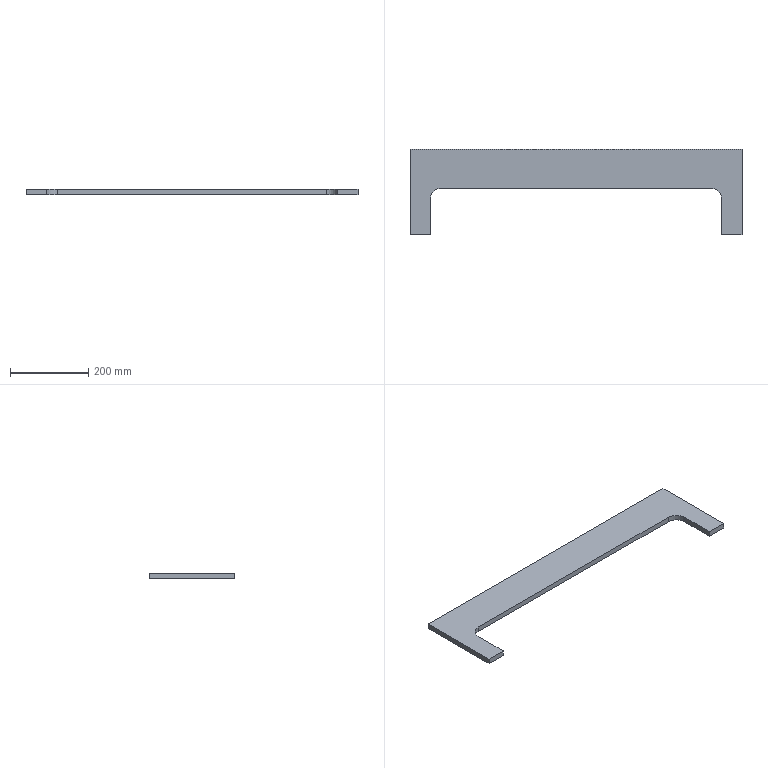Part | STEP file | 2012-06-08-04 | 1 solid | 12 faces | box 850 x 220 x 14 mm | volume 1368448 mm3 | plane 10 | cylinder 2 | commonest cylinder face diameters 60 x2
STEP:
#1=CARTESIAN_POINT('',(0.,0.,0.));
#2=DIRECTION('',(0.,0.,1.));
#3=DIRECTION('',(1.,0.,0.));
#4=AXIS2_PLACEMENT_3D('',#1,#2,#3);
#5=CARTESIAN_POINT('',(-425.,-110.,0.));
#6=VERTEX_POINT('',#5);
#7=CARTESIAN_POINT('',(-373.5,-110.,0.));
#8=VERTEX_POINT('',#7);
#9=CARTESIAN_POINT('',(-425.,-110.,0.));
#10=DIRECTION('',(1.,0.,0.));
#11=VECTOR('',#10,1.);
#12=LINE('',#9,#11);
#13=CARTESIAN_POINT('',(-425.,-110.,14.));
#14=DIRECTION('',(0.,1.,0.));
#15=DIRECTION('',(0.,0.,1.));
#16=AXIS2_PLACEMENT_3D('',#13,#14,#15);
#17=PLANE('',#16);
#18=CARTESIAN_POINT('',(-14.,0.));
#19=DIRECTION('',(0.,1.));
#20=VECTOR('',#19,1.);
#21=LINE('',#18,#20);
#22=(GEOMETRIC_REPRESENTATION_CONTEXT(2)PARAMETRIC_REPRESENTATION_CONTEXT()REPRESENTATION_CONTEXT('',''));
#23=DEFINITIONAL_REPRESENTATION('',(#21),#22);
#24=PCURVE('',#17,#23);
#25=CARTESIAN_POINT('',(425.,-110.,0.));
#26=DIRECTION('',(0.,0.,1.));
#27=DIRECTION('',(1.,0.,0.));
#28=AXIS2_PLACEMENT_3D('',#25,#26,#27);
#29=PLANE('',#28);
#30=CARTESIAN_POINT('',(-850.,0.));
#31=DIRECTION('',(1.,0.));
#32=VECTOR('',#31,1.);
#33=LINE('',#30,#32);
#34=(GEOMETRIC_REPRESENTATION_CONTEXT(2)PARAMETRIC_REPRESENTATION_CONTEXT()REPRESENTATION_CONTEXT('',''));
#35=DEFINITIONAL_REPRESENTATION('',(#33),#34);
#36=PCURVE('',#29,#35);
#37=SURFACE_CURVE('',#12,(#24,#36),.PCURVE_S1.);
#38=EDGE_CURVE('',#6,#8,#37,.T.);
#39=ORIENTED_EDGE('',*,*,#38,.T.);
#40=CARTESIAN_POINT('',(-373.5,-110.,14.));
#41=VERTEX_POINT('',#40);
#42=CARTESIAN_POINT('',(-373.5,-110.,0.));
#43=DIRECTION('',(0.,0.,1.));
#44=VECTOR('',#43,1.);
#45=LINE('',#42,#44);
#46=CARTESIAN_POINT('',(-14.,51.5));
#47=DIRECTION('',(1.,0.));
#48=VECTOR('',#47,1.);
#49=LINE('',#46,#48);
#50=(GEOMETRIC_REPRESENTATION_CONTEXT(2)PARAMETRIC_REPRESENTATION_CONTEXT()REPRESENTATION_CONTEXT('',''));
#51=DEFINITIONAL_REPRESENTATION('',(#49),#50);
#52=PCURVE('',#17,#51);
#53=CARTESIAN_POINT('',(-373.5,-110.,0.));
#54=DIRECTION('',(-1.,0.,0.));
#55=DIRECTION('',(0.,0.,1.));
#56=AXIS2_PLACEMENT_3D('',#53,#54,#55);
#57=PLANE('',#56);
#58=CARTESIAN_POINT('',(0.,0.));
#59=DIRECTION('',(1.,0.));
#60=VECTOR('',#59,1.);
#61=LINE('',#58,#60);
#62=(GEOMETRIC_REPRESENTATION_CONTEXT(2)PARAMETRIC_REPRESENTATION_CONTEXT()REPRESENTATION_CONTEXT('',''));
#63=DEFINITIONAL_REPRESENTATION('',(#61),#62);
#64=PCURVE('',#57,#63);
#65=SURFACE_CURVE('',#45,(#52,#64),.PCURVE_S1.);
#66=EDGE_CURVE('',#8,#41,#65,.T.);
#67=ORIENTED_EDGE('',*,*,#66,.T.);
#68=CARTESIAN_POINT('',(-425.,-110.,14.));
#69=VERTEX_POINT('',#68);
#70=CARTESIAN_POINT('',(-425.,-110.,14.));
#71=DIRECTION('',(1.,0.,0.));
#72=VECTOR('',#71,1.);
#73=LINE('',#70,#72);
#74=CARTESIAN_POINT('',(0.,0.));
#75=DIRECTION('',(0.,1.));
#76=VECTOR('',#75,1.);
#77=LINE('',#74,#76);
#78=(GEOMETRIC_REPRESENTATION_CONTEXT(2)PARAMETRIC_REPRESENTATION_CONTEXT()REPRESENTATION_CONTEXT('',''));
#79=DEFINITIONAL_REPRESENTATION('',(#77),#78);
#80=PCURVE('',#17,#79);
#81=CARTESIAN_POINT('',(425.,-110.,14.));
#82=DIRECTION('',(0.,0.,1.));
#83=DIRECTION('',(1.,0.,0.));
#84=AXIS2_PLACEMENT_3D('',#81,#82,#83);
#85=PLANE('',#84);
#86=CARTESIAN_POINT('',(-850.,0.));
#87=DIRECTION('',(1.,0.));
#88=VECTOR('',#87,1.);
#89=LINE('',#86,#88);
#90=(GEOMETRIC_REPRESENTATION_CONTEXT(2)PARAMETRIC_REPRESENTATION_CONTEXT()REPRESENTATION_CONTEXT('',''));
#91=DEFINITIONAL_REPRESENTATION('',(#89),#90);
#92=PCURVE('',#85,#91);
#93=SURFACE_CURVE('',#73,(#80,#92),.PCURVE_S1.);
#94=EDGE_CURVE('',#69,#41,#93,.T.);
#95=ORIENTED_EDGE('',*,*,#94,.F.);
#96=CARTESIAN_POINT('',(-425.,-110.,14.));
#97=DIRECTION('',(0.,0.,-1.));
#98=VECTOR('',#97,1.);
#99=LINE('',#96,#98);
#100=CARTESIAN_POINT('',(0.,0.));
#101=DIRECTION('',(-1.,0.));
#102=VECTOR('',#101,1.);
#103=LINE('',#100,#102);
#104=(GEOMETRIC_REPRESENTATION_CONTEXT(2)PARAMETRIC_REPRESENTATION_CONTEXT()REPRESENTATION_CONTEXT('',''));
#105=DEFINITIONAL_REPRESENTATION('',(#103),#104);
#106=PCURVE('',#17,#105);
#107=CARTESIAN_POINT('',(-425.,110.,14.));
#108=DIRECTION('',(1.,0.,0.));
#109=DIRECTION('',(0.,1.,0.));
#110=AXIS2_PLACEMENT_3D('',#107,#108,#109);
#111=PLANE('',#110);
#112=CARTESIAN_POINT('',(-220.,0.));
#113=DIRECTION('',(0.,-1.));
#114=VECTOR('',#113,1.);
#115=LINE('',#112,#114);
#116=(GEOMETRIC_REPRESENTATION_CONTEXT(2)PARAMETRIC_REPRESENTATION_CONTEXT()REPRESENTATION_CONTEXT('',''));
#117=DEFINITIONAL_REPRESENTATION('',(#115),#116);
#118=PCURVE('',#111,#117);
#119=SURFACE_CURVE('',#99,(#106,#118),.PCURVE_S1.);
#120=EDGE_CURVE('',#69,#6,#119,.T.);
#121=ORIENTED_EDGE('',*,*,#120,.T.);
#122=EDGE_LOOP('',(#39,#67,#95,#121));
#123=FACE_BOUND('',#122,.T.);
#124=ADVANCED_FACE('',(#123),#17,.F.);
#125=CARTESIAN_POINT('',(425.,-110.,0.));
#126=VERTEX_POINT('',#125);
#127=CARTESIAN_POINT('',(425.,110.,0.));
#128=VERTEX_POINT('',#127);
#129=CARTESIAN_POINT('',(425.,110.,0.));
#130=DIRECTION('',(0.,1.,0.));
#131=VECTOR('',#130,1.);
#132=LINE('',#129,#131);
#133=CARTESIAN_POINT('',(425.,110.,14.));
#134=DIRECTION('',(-1.,0.,0.));
#135=DIRECTION('',(0.,0.,1.));
#136=AXIS2_PLACEMENT_3D('',#133,#134,#135);
#137=PLANE('',#136);
#138=CARTESIAN_POINT('',(-14.,0.));
#139=DIRECTION('',(0.,1.));
#140=VECTOR('',#139,1.);
#141=LINE('',#138,#140);
#142=(GEOMETRIC_REPRESENTATION_CONTEXT(2)PARAMETRIC_REPRESENTATION_CONTEXT()REPRESENTATION_CONTEXT('',''));
#143=DEFINITIONAL_REPRESENTATION('',(#141),#142);
#144=PCURVE('',#137,#143);
#145=CARTESIAN_POINT('',(0.,220.));
#146=DIRECTION('',(0.,1.));
#147=VECTOR('',#146,1.);
#148=LINE('',#145,#147);
#149=(GEOMETRIC_REPRESENTATION_CONTEXT(2)PARAMETRIC_REPRESENTATION_CONTEXT()REPRESENTATION_CONTEXT('',''));
#150=DEFINITIONAL_REPRESENTATION('',(#148),#149);
#151=PCURVE('',#29,#150);
#152=SURFACE_CURVE('',#132,(#144,#151),.PCURVE_S1.);
#153=EDGE_CURVE('',#126,#128,#152,.T.);
#154=ORIENTED_EDGE('',*,*,#153,.T.);
#155=CARTESIAN_POINT('',(425.,110.,14.));
#156=VERTEX_POINT('',#155);
#157=CARTESIAN_POINT('',(425.,110.,14.));
#158=DIRECTION('',(0.,0.,-1.));
#159=VECTOR('',#158,1.);
#160=LINE('',#157,#159);
#161=CARTESIAN_POINT('',(0.,0.));
#162=DIRECTION('',(-1.,0.));
#163=VECTOR('',#162,1.);
#164=LINE('',#161,#163);
#165=(GEOMETRIC_REPRESENTATION_CONTEXT(2)PARAMETRIC_REPRESENTATION_CONTEXT()REPRESENTATION_CONTEXT('',''));
#166=DEFINITIONAL_REPRESENTATION('',(#164),#165);
#167=PCURVE('',#137,#166);
#168=CARTESIAN_POINT('',(-425.,110.,14.));
#169=DIRECTION('',(0.,-1.,0.));
#170=DIRECTION('',(0.,0.,-1.));
#171=AXIS2_PLACEMENT_3D('',#168,#169,#170);
#172=PLANE('',#171);
#173=CARTESIAN_POINT('',(0.,850.));
#174=DIRECTION('',(1.,0.));
#175=VECTOR('',#174,1.);
#176=LINE('',#173,#175);
#177=(GEOMETRIC_REPRESENTATION_CONTEXT(2)PARAMETRIC_REPRESENTATION_CONTEXT()REPRESENTATION_CONTEXT('',''));
#178=DEFINITIONAL_REPRESENTATION('',(#176),#177);
#179=PCURVE('',#172,#178);
#180=SURFACE_CURVE('',#160,(#167,#179),.PCURVE_S1.);
#181=EDGE_CURVE('',#156,#128,#180,.T.);
#182=ORIENTED_EDGE('',*,*,#181,.F.);
#183=CARTESIAN_POINT('',(425.,-110.,14.));
#184=VERTEX_POINT('',#183);
#185=CARTESIAN_POINT('',(425.,110.,14.));
#186=DIRECTION('',(0.,1.,0.));
#187=VECTOR('',#186,1.);
#188=LINE('',#185,#187);
#189=CARTESIAN_POINT('',(0.,0.));
#190=DIRECTION('',(0.,1.));
#191=VECTOR('',#190,1.);
#192=LINE('',#189,#191);
#193=(GEOMETRIC_REPRESENTATION_CONTEXT(2)PARAMETRIC_REPRESENTATION_CONTEXT()REPRESENTATION_CONTEXT('',''));
#194=DEFINITIONAL_REPRESENTATION('',(#192),#193);
#195=PCURVE('',#137,#194);
#196=CARTESIAN_POINT('',(0.,220.));
#197=DIRECTION('',(0.,1.));
#198=VECTOR('',#197,1.);
#199=LINE('',#196,#198);
#200=(GEOMETRIC_REPRESENTATION_CONTEXT(2)PARAMETRIC_REPRESENTATION_CONTEXT()REPRESENTATION_CONTEXT('',''));
#201=DEFINITIONAL_REPRESENTATION('',(#199),#200);
#202=PCURVE('',#85,#201);
#203=SURFACE_CURVE('',#188,(#195,#202),.PCURVE_S1.);
#204=EDGE_CURVE('',#184,#156,#203,.T.);
#205=ORIENTED_EDGE('',*,*,#204,.F.);
#206=CARTESIAN_POINT('',(425.,-110.,14.));
#207=DIRECTION('',(0.,0.,-1.));
#208=VECTOR('',#207,1.);
#209=LINE('',#206,#208);
#210=CARTESIAN_POINT('',(0.,-220.));
#211=DIRECTION('',(-1.,0.));
#212=VECTOR('',#211,1.);
#213=LINE('',#210,#212);
#214=(GEOMETRIC_REPRESENTATION_CONTEXT(2)PARAMETRIC_REPRESENTATION_CONTEXT()REPRESENTATION_CONTEXT('',''));
#215=DEFINITIONAL_REPRESENTATION('',(#213),#214);
#216=PCURVE('',#137,#215);
#217=CARTESIAN_POINT('',(-425.,-110.,14.));
#218=DIRECTION('',(0.,1.,0.));
#219=DIRECTION('',(0.,0.,1.));
#220=AXIS2_PLACEMENT_3D('',#217,#218,#219);
#221=PLANE('',#220);
#222=CARTESIAN_POINT('',(0.,850.));
#223=DIRECTION('',(-1.,0.));
#224=VECTOR('',#223,1.);
#225=LINE('',#222,#224);
#226=(GEOMETRIC_REPRESENTATION_CONTEXT(2)PARAMETRIC_REPRESENTATION_CONTEXT()REPRESENTATION_CONTEXT('',''));
#227=DEFINITIONAL_REPRESENTATION('',(#225),#226);
#228=PCURVE('',#221,#227);
#229=SURFACE_CURVE('',#209,(#216,#228),.PCURVE_S1.);
#230=EDGE_CURVE('',#184,#126,#229,.T.);
#231=ORIENTED_EDGE('',*,*,#230,.T.);
#232=EDGE_LOOP('',(#154,#182,#205,#231));
#233=FACE_BOUND('',#232,.T.);
#234=ADVANCED_FACE('',(#233),#137,.F.);
#235=CARTESIAN_POINT('',(-425.,110.,0.));
#236=VERTEX_POINT('',#235);
#237=CARTESIAN_POINT('',(-425.,110.,0.));
#238=DIRECTION('',(-1.,0.,0.));
#239=VECTOR('',#238,1.);
#240=LINE('',#237,#239);
#241=CARTESIAN_POINT('',(14.,0.));
#242=DIRECTION('',(0.,-1.));
#243=VECTOR('',#242,1.);
#244=LINE('',#241,#243);
#245=(GEOMETRIC_REPRESENTATION_CONTEXT(2)PARAMETRIC_REPRESENTATION_CONTEXT()REPRESENTATION_CONTEXT('',''));
#246=DEFINITIONAL_REPRESENTATION('',(#244),#245);
#247=PCURVE('',#172,#246);
#248=CARTESIAN_POINT('',(-850.,220.));
#249=DIRECTION('',(-1.,0.));
#250=VECTOR('',#249,1.);
#251=LINE('',#248,#250);
#252=(GEOMETRIC_REPRESENTATION_CONTEXT(2)PARAMETRIC_REPRESENTATION_CONTEXT()REPRESENTATION_CONTEXT('',''));
#253=DEFINITIONAL_REPRESENTATION('',(#251),#252);
#254=PCURVE('',#29,#253);
#255=SURFACE_CURVE('',#240,(#247,#254),.PCURVE_S1.);
#256=EDGE_CURVE('',#128,#236,#255,.T.);
#257=ORIENTED_EDGE('',*,*,#256,.T.);
#258=CARTESIAN_POINT('',(-425.,110.,14.));
#259=VERTEX_POINT('',#258);
#260=CARTESIAN_POINT('',(-425.,110.,14.));
#261=DIRECTION('',(0.,0.,-1.));
#262=VECTOR('',#261,1.);
#263=LINE('',#260,#262);
#264=CARTESIAN_POINT('',(0.,0.));
#265=DIRECTION('',(1.,0.));
#266=VECTOR('',#265,1.);
#267=LINE('',#264,#266);
#268=(GEOMETRIC_REPRESENTATION_CONTEXT(2)PARAMETRIC_REPRESENTATION_CONTEXT()REPRESENTATION_CONTEXT('',''));
#269=DEFINITIONAL_REPRESENTATION('',(#267),#268);
#270=PCURVE('',#172,#269);
#271=CARTESIAN_POINT('',(0.,0.));
#272=DIRECTION('',(0.,-1.));
#273=VECTOR('',#272,1.);
#274=LINE('',#271,#273);
#275=(GEOMETRIC_REPRESENTATION_CONTEXT(2)PARAMETRIC_REPRESENTATION_CONTEXT()REPRESENTATION_CONTEXT('',''));
#276=DEFINITIONAL_REPRESENTATION('',(#274),#275);
#277=PCURVE('',#111,#276);
#278=SURFACE_CURVE('',#263,(#270,#277),.PCURVE_S1.);
#279=EDGE_CURVE('',#259,#236,#278,.T.);
#280=ORIENTED_EDGE('',*,*,#279,.F.);
#281=CARTESIAN_POINT('',(-425.,110.,14.));
#282=DIRECTION('',(-1.,0.,0.));
#283=VECTOR('',#282,1.);
#284=LINE('',#281,#283);
#285=CARTESIAN_POINT('',(0.,0.));
#286=DIRECTION('',(0.,-1.));
#287=VECTOR('',#286,1.);
#288=LINE('',#285,#287);
#289=(GEOMETRIC_REPRESENTATION_CONTEXT(2)PARAMETRIC_REPRESENTATION_CONTEXT()REPRESENTATION_CONTEXT('',''));
#290=DEFINITIONAL_REPRESENTATION('',(#288),#289);
#291=PCURVE('',#172,#290);
#292=CARTESIAN_POINT('',(-850.,220.));
#293=DIRECTION('',(-1.,0.));
#294=VECTOR('',#293,1.);
#295=LINE('',#292,#294);
#296=(GEOMETRIC_REPRESENTATION_CONTEXT(2)PARAMETRIC_REPRESENTATION_CONTEXT()REPRESENTATION_CONTEXT('',''));
#297=DEFINITIONAL_REPRESENTATION('',(#295),#296);
#298=PCURVE('',#85,#297);
#299=SURFACE_CURVE('',#284,(#291,#298),.PCURVE_S1.);
#300=EDGE_CURVE('',#156,#259,#299,.T.);
#301=ORIENTED_EDGE('',*,*,#300,.F.);
#302=ORIENTED_EDGE('',*,*,#181,.T.);
#303=EDGE_LOOP('',(#257,#280,#301,#302));
#304=FACE_BOUND('',#303,.T.);
#305=ADVANCED_FACE('',(#304),#172,.F.);
#306=CARTESIAN_POINT('',(-425.,110.,0.));
#307=DIRECTION('',(0.,-1.,0.));
#308=VECTOR('',#307,1.);
#309=LINE('',#306,#308);
#310=CARTESIAN_POINT('',(0.,-14.));
#311=DIRECTION('',(-1.,0.));
#312=VECTOR('',#311,1.);
#313=LINE('',#310,#312);
#314=(GEOMETRIC_REPRESENTATION_CONTEXT(2)PARAMETRIC_REPRESENTATION_CONTEXT()REPRESENTATION_CONTEXT('',''));
#315=DEFINITIONAL_REPRESENTATION('',(#313),#314);
#316=PCURVE('',#111,#315);
#317=CARTESIAN_POINT('',(-850.,220.));
#318=DIRECTION('',(0.,-1.));
#319=VECTOR('',#318,1.);
#320=LINE('',#317,#319);
#321=(GEOMETRIC_REPRESENTATION_CONTEXT(2)PARAMETRIC_REPRESENTATION_CONTEXT()REPRESENTATION_CONTEXT('',''));
#322=DEFINITIONAL_REPRESENTATION('',(#320),#321);
#323=PCURVE('',#29,#322);
#324=SURFACE_CURVE('',#309,(#316,#323),.PCURVE_S1.);
#325=EDGE_CURVE('',#236,#6,#324,.T.);
#326=ORIENTED_EDGE('',*,*,#325,.T.);
#327=ORIENTED_EDGE('',*,*,#120,.F.);
#328=CARTESIAN_POINT('',(-425.,110.,14.));
#329=DIRECTION('',(0.,-1.,0.));
#330=VECTOR('',#329,1.);
#331=LINE('',#328,#330);
#332=CARTESIAN_POINT('',(0.,0.));
#333=DIRECTION('',(-1.,0.));
#334=VECTOR('',#333,1.);
#335=LINE('',#332,#334);
#336=(GEOMETRIC_REPRESENTATION_CONTEXT(2)PARAMETRIC_REPRESENTATION_CONTEXT()REPRESENTATION_CONTEXT('',''));
#337=DEFINITIONAL_REPRESENTATION('',(#335),#336);
#338=PCURVE('',#111,#337);
#339=CARTESIAN_POINT('',(-850.,220.));
#340=DIRECTION('',(0.,-1.));
#341=VECTOR('',#340,1.);
#342=LINE('',#339,#341);
#343=(GEOMETRIC_REPRESENTATION_CONTEXT(2)PARAMETRIC_REPRESENTATION_CONTEXT()REPRESENTATION_CONTEXT('',''));
#344=DEFINITIONAL_REPRESENTATION('',(#342),#343);
#345=PCURVE('',#85,#344);
#346=SURFACE_CURVE('',#331,(#338,#345),.PCURVE_S1.);
#347=EDGE_CURVE('',#259,#69,#346,.T.);
#348=ORIENTED_EDGE('',*,*,#347,.F.);
#349=ORIENTED_EDGE('',*,*,#279,.T.);
#350=EDGE_LOOP('',(#326,#327,#348,#349));
#351=FACE_BOUND('',#350,.T.);
#352=ADVANCED_FACE('',(#351),#111,.F.);
#353=CARTESIAN_POINT('',(373.5,-110.,14.));
#354=VERTEX_POINT('',#353);
#355=CARTESIAN_POINT('',(-425.,-110.,14.));
#356=DIRECTION('',(1.,0.,0.));
#357=VECTOR('',#356,1.);
#358=LINE('',#355,#357);
#359=CARTESIAN_POINT('',(0.,0.));
#360=DIRECTION('',(0.,1.));
#361=VECTOR('',#360,1.);
#362=LINE('',#359,#361);
#363=(GEOMETRIC_REPRESENTATION_CONTEXT(2)PARAMETRIC_REPRESENTATION_CONTEXT()REPRESENTATION_CONTEXT('',''));
#364=DEFINITIONAL_REPRESENTATION('',(#362),#363);
#365=PCURVE('',#221,#364);
#366=CARTESIAN_POINT('',(-850.,0.));
#367=DIRECTION('',(1.,0.));
#368=VECTOR('',#367,1.);
#369=LINE('',#366,#368);
#370=(GEOMETRIC_REPRESENTATION_CONTEXT(2)PARAMETRIC_REPRESENTATION_CONTEXT()REPRESENTATION_CONTEXT('',''));
#371=DEFINITIONAL_REPRESENTATION('',(#369),#370);
#372=PCURVE('',#85,#371);
#373=SURFACE_CURVE('',#358,(#365,#372),.PCURVE_S1.);
#374=EDGE_CURVE('',#354,#184,#373,.T.);
#375=ORIENTED_EDGE('',*,*,#374,.F.);
#376=CARTESIAN_POINT('',(373.5,-110.,0.));
#377=VERTEX_POINT('',#376);
#378=CARTESIAN_POINT('',(373.5,-110.,0.));
#379=DIRECTION('',(0.,0.,1.));
#380=VECTOR('',#379,1.);
#381=LINE('',#378,#380);
#382=CARTESIAN_POINT('',(-14.,798.5));
#383=DIRECTION('',(1.,0.));
#384=VECTOR('',#383,1.);
#385=LINE('',#382,#384);
#386=(GEOMETRIC_REPRESENTATION_CONTEXT(2)PARAMETRIC_REPRESENTATION_CONTEXT()REPRESENTATION_CONTEXT('',''));
#387=DEFINITIONAL_REPRESENTATION('',(#385),#386);
#388=PCURVE('',#221,#387);
#389=CARTESIAN_POINT('',(373.5,-110.,0.));
#390=DIRECTION('',(1.,0.,0.));
#391=DIRECTION('',(0.,1.,0.));
#392=AXIS2_PLACEMENT_3D('',#389,#390,#391);
#393=PLANE('',#392);
#394=CARTESIAN_POINT('',(0.,0.));
#395=DIRECTION('',(0.,1.));
#396=VECTOR('',#395,1.);
#397=LINE('',#394,#396);
#398=(GEOMETRIC_REPRESENTATION_CONTEXT(2)PARAMETRIC_REPRESENTATION_CONTEXT()REPRESENTATION_CONTEXT('',''));
#399=DEFINITIONAL_REPRESENTATION('',(#397),#398);
#400=PCURVE('',#393,#399);
#401=SURFACE_CURVE('',#381,(#388,#400),.PCURVE_S1.);
#402=EDGE_CURVE('',#377,#354,#401,.T.);
#403=ORIENTED_EDGE('',*,*,#402,.F.);
#404=CARTESIAN_POINT('',(-425.,-110.,0.));
#405=DIRECTION('',(1.,0.,0.));
#406=VECTOR('',#405,1.);
#407=LINE('',#404,#406);
#408=CARTESIAN_POINT('',(-14.,0.));
#409=DIRECTION('',(0.,1.));
#410=VECTOR('',#409,1.);
#411=LINE('',#408,#410);
#412=(GEOMETRIC_REPRESENTATION_CONTEXT(2)PARAMETRIC_REPRESENTATION_CONTEXT()REPRESENTATION_CONTEXT('',''));
#413=DEFINITIONAL_REPRESENTATION('',(#411),#412);
#414=PCURVE('',#221,#413);
#415=CARTESIAN_POINT('',(-850.,0.));
#416=DIRECTION('',(1.,0.));
#417=VECTOR('',#416,1.);
#418=LINE('',#415,#417);
#419=(GEOMETRIC_REPRESENTATION_CONTEXT(2)PARAMETRIC_REPRESENTATION_CONTEXT()REPRESENTATION_CONTEXT('',''));
#420=DEFINITIONAL_REPRESENTATION('',(#418),#419);
#421=PCURVE('',#29,#420);
#422=SURFACE_CURVE('',#407,(#414,#421),.PCURVE_S1.);
#423=EDGE_CURVE('',#377,#126,#422,.T.);
#424=ORIENTED_EDGE('',*,*,#423,.T.);
#425=ORIENTED_EDGE('',*,*,#230,.F.);
#426=EDGE_LOOP('',(#375,#403,#424,#425));
#427=FACE_BOUND('',#426,.T.);
#428=ADVANCED_FACE('',(#427),#221,.F.);
#429=CARTESIAN_POINT('',(-373.5,-20.,14.));
#430=VERTEX_POINT('',#429);
#431=CARTESIAN_POINT('',(-373.5,-110.,14.));
#432=DIRECTION('',(0.,-1.,0.));
#433=VECTOR('',#432,1.);
#434=LINE('',#431,#433);
#435=CARTESIAN_POINT('',(-798.5,0.));
#436=DIRECTION('',(0.,-1.));
#437=VECTOR('',#436,1.);
#438=LINE('',#435,#437);
#439=(GEOMETRIC_REPRESENTATION_CONTEXT(2)PARAMETRIC_REPRESENTATION_CONTEXT()REPRESENTATION_CONTEXT('',''));
#440=DEFINITIONAL_REPRESENTATION('',(#438),#439);
#441=PCURVE('',#85,#440);
#442=CARTESIAN_POINT('',(14.,0.));
#443=DIRECTION('',(0.,-1.));
#444=VECTOR('',#443,1.);
#445=LINE('',#442,#444);
#446=(GEOMETRIC_REPRESENTATION_CONTEXT(2)PARAMETRIC_REPRESENTATION_CONTEXT()REPRESENTATION_CONTEXT('',''));
#447=DEFINITIONAL_REPRESENTATION('',(#445),#446);
#448=PCURVE('',#57,#447);
#449=SURFACE_CURVE('',#434,(#441,#448),.PCURVE_S1.);
#450=EDGE_CURVE('',#430,#41,#449,.T.);
#451=ORIENTED_EDGE('',*,*,#450,.F.);
#452=CARTESIAN_POINT('',(-343.5,10.,14.));
#453=VERTEX_POINT('',#452);
#454=CARTESIAN_POINT('',(-343.5,-20.,14.));
#455=DIRECTION('',(0.,0.,-1.));
#456=DIRECTION('',(1.,0.,0.));
#457=AXIS2_PLACEMENT_3D('',#454,#455,#456);
#458=CIRCLE('',#457,30.);
#459=CARTESIAN_POINT('',(-738.5,90.));
#460=CARTESIAN_POINT('',(-738.5,38.038));
#461=CARTESIAN_POINT('',(-783.5,64.019));
#462=CARTESIAN_POINT('',(-828.5,90.));
#463=CARTESIAN_POINT('',(-783.5,115.981));
#464=CARTESIAN_POINT('',(-738.5,141.962));
#465=CARTESIAN_POINT('',(-738.5,90.));
#466=(BOUNDED_CURVE()B_SPLINE_CURVE(2,(#459,#460,#461,#462,#463,#464,#465),.UNSPECIFIED.,.T.,.F.)B_SPLINE_CURVE_WITH_KNOTS((1,2,2,2,2,1),(-2.094,0.,2.094,4.189,6.283,8.378),.UNSPECIFIED.)CURVE()GEOMETRIC_REPRESENTATION_ITEM()RATIONAL_B_SPLINE_CURVE((1.,0.5,1.,0.5,1.,0.5,1.))REPRESENTATION_ITEM(''));
#467=(GEOMETRIC_REPRESENTATION_CONTEXT(2)PARAMETRIC_REPRESENTATION_CONTEXT()REPRESENTATION_CONTEXT('',''));
#468=DEFINITIONAL_REPRESENTATION('',(#466),#467);
#469=PCURVE('',#85,#468);
#470=CARTESIAN_POINT('',(-343.5,-20.,0.));
#471=DIRECTION('',(0.,0.,-1.));
#472=DIRECTION('',(-1.,0.,0.));
#473=AXIS2_PLACEMENT_3D('',#470,#471,#472);
#474=CYLINDRICAL_SURFACE('',#473,30.);
#475=CARTESIAN_POINT('',(-3.142,-14.));
#476=DIRECTION('',(1.,0.));
#477=VECTOR('',#476,1.);
#478=LINE('',#475,#477);
#479=(GEOMETRIC_REPRESENTATION_CONTEXT(2)PARAMETRIC_REPRESENTATION_CONTEXT()REPRESENTATION_CONTEXT('',''));
#480=DEFINITIONAL_REPRESENTATION('',(#478),#479);
#481=PCURVE('',#474,#480);
#482=SURFACE_CURVE('',#458,(#469,#481),.PCURVE_S1.);
#483=EDGE_CURVE('',#430,#453,#482,.T.);
#484=ORIENTED_EDGE('',*,*,#483,.T.);
#485=CARTESIAN_POINT('',(343.5,10.,14.));
#486=VERTEX_POINT('',#485);
#487=CARTESIAN_POINT('',(-373.5,10.,14.));
#488=DIRECTION('',(-1.,0.,0.));
#489=VECTOR('',#488,1.);
#490=LINE('',#487,#489);
#491=CARTESIAN_POINT('',(-798.5,120.));
#492=DIRECTION('',(-1.,0.));
#493=VECTOR('',#492,1.);
#494=LINE('',#491,#493);
#495=(GEOMETRIC_REPRESENTATION_CONTEXT(2)PARAMETRIC_REPRESENTATION_CONTEXT()REPRESENTATION_CONTEXT('',''));
#496=DEFINITIONAL_REPRESENTATION('',(#494),#495);
#497=PCURVE('',#85,#496);
#498=CARTESIAN_POINT('',(-373.5,10.,0.));
#499=DIRECTION('',(0.,1.,0.));
#500=DIRECTION('',(-1.,0.,0.));
#501=AXIS2_PLACEMENT_3D('',#498,#499,#500);
#502=PLANE('',#501);
#503=CARTESIAN_POINT('',(0.,14.));
#504=DIRECTION('',(1.,0.));
#505=VECTOR('',#504,1.);
#506=LINE('',#503,#505);
#507=(GEOMETRIC_REPRESENTATION_CONTEXT(2)PARAMETRIC_REPRESENTATION_CONTEXT()REPRESENTATION_CONTEXT('',''));
#508=DEFINITIONAL_REPRESENTATION('',(#506),#507);
#509=PCURVE('',#502,#508);
#510=SURFACE_CURVE('',#490,(#497,#509),.PCURVE_S1.);
#511=EDGE_CURVE('',#486,#453,#510,.T.);
#512=ORIENTED_EDGE('',*,*,#511,.F.);
#513=CARTESIAN_POINT('',(373.5,-20.,14.));
#514=VERTEX_POINT('',#513);
#515=CARTESIAN_POINT('',(343.5,-20.,14.));
#516=DIRECTION('',(0.,0.,-1.));
#517=DIRECTION('',(1.,0.,0.));
#518=AXIS2_PLACEMENT_3D('',#515,#516,#517);
#519=CIRCLE('',#518,30.);
#520=CARTESIAN_POINT('',(-51.5,90.));
#521=CARTESIAN_POINT('',(-51.5,38.038));
#522=CARTESIAN_POINT('',(-96.5,64.019));
#523=CARTESIAN_POINT('',(-141.5,90.));
#524=CARTESIAN_POINT('',(-96.5,115.981));
#525=CARTESIAN_POINT('',(-51.5,141.962));
#526=CARTESIAN_POINT('',(-51.5,90.));
#527=(BOUNDED_CURVE()B_SPLINE_CURVE(2,(#520,#521,#522,#523,#524,#525,#526),.UNSPECIFIED.,.T.,.F.)B_SPLINE_CURVE_WITH_KNOTS((1,2,2,2,2,1),(-2.094,0.,2.094,4.189,6.283,8.378),.UNSPECIFIED.)CURVE()GEOMETRIC_REPRESENTATION_ITEM()RATIONAL_B_SPLINE_CURVE((1.,0.5,1.,0.5,1.,0.5,1.))REPRESENTATION_ITEM(''));
#528=(GEOMETRIC_REPRESENTATION_CONTEXT(2)PARAMETRIC_REPRESENTATION_CONTEXT()REPRESENTATION_CONTEXT('',''));
#529=DEFINITIONAL_REPRESENTATION('',(#527),#528);
#530=PCURVE('',#85,#529);
#531=CARTESIAN_POINT('',(343.5,-20.,0.));
#532=DIRECTION('',(0.,0.,-1.));
#533=DIRECTION('',(-1.,0.,0.));
#534=AXIS2_PLACEMENT_3D('',#531,#532,#533);
#535=CYLINDRICAL_SURFACE('',#534,30.);
#536=CARTESIAN_POINT('',(-3.142,-14.));
#537=DIRECTION('',(1.,0.));
#538=VECTOR('',#537,1.);
#539=LINE('',#536,#538);
#540=(GEOMETRIC_REPRESENTATION_CONTEXT(2)PARAMETRIC_REPRESENTATION_CONTEXT()REPRESENTATION_CONTEXT('',''));
#541=DEFINITIONAL_REPRESENTATION('',(#539),#540);
#542=PCURVE('',#535,#541);
#543=SURFACE_CURVE('',#519,(#530,#542),.PCURVE_S1.);
#544=EDGE_CURVE('',#486,#514,#543,.T.);
#545=ORIENTED_EDGE('',*,*,#544,.T.);
#546=CARTESIAN_POINT('',(373.5,-110.,14.));
#547=DIRECTION('',(0.,1.,0.));
#548=VECTOR('',#547,1.);
#549=LINE('',#546,#548);
#550=CARTESIAN_POINT('',(-51.5,0.));
#551=DIRECTION('',(0.,1.));
#552=VECTOR('',#551,1.);
#553=LINE('',#550,#552);
#554=(GEOMETRIC_REPRESENTATION_CONTEXT(2)PARAMETRIC_REPRESENTATION_CONTEXT()REPRESENTATION_CONTEXT('',''));
#555=DEFINITIONAL_REPRESENTATION('',(#553),#554);
#556=PCURVE('',#85,#555);
#557=CARTESIAN_POINT('',(0.,14.));
#558=DIRECTION('',(1.,0.));
#559=VECTOR('',#558,1.);
#560=LINE('',#557,#559);
#561=(GEOMETRIC_REPRESENTATION_CONTEXT(2)PARAMETRIC_REPRESENTATION_CONTEXT()REPRESENTATION_CONTEXT('',''));
#562=DEFINITIONAL_REPRESENTATION('',(#560),#561);
#563=PCURVE('',#393,#562);
#564=SURFACE_CURVE('',#549,(#556,#563),.PCURVE_S1.);
#565=EDGE_CURVE('',#354,#514,#564,.T.);
#566=ORIENTED_EDGE('',*,*,#565,.F.);
#567=ORIENTED_EDGE('',*,*,#374,.T.);
#568=ORIENTED_EDGE('',*,*,#204,.T.);
#569=ORIENTED_EDGE('',*,*,#300,.T.);
#570=ORIENTED_EDGE('',*,*,#347,.T.);
#571=ORIENTED_EDGE('',*,*,#94,.T.);
#572=EDGE_LOOP('',(#451,#484,#512,#545,#566,#567,#568,#569,#570,#571));
#573=FACE_BOUND('',#572,.T.);
#574=ADVANCED_FACE('',(#573),#85,.T.);
#575=CARTESIAN_POINT('',(373.5,-20.,0.));
#576=VERTEX_POINT('',#575);
#577=CARTESIAN_POINT('',(373.5,-110.,0.));
#578=DIRECTION('',(0.,1.,0.));
#579=VECTOR('',#578,1.);
#580=LINE('',#577,#579);
#581=CARTESIAN_POINT('',(-51.5,0.));
#582=DIRECTION('',(0.,1.));
#583=VECTOR('',#582,1.);
#584=LINE('',#581,#583);
#585=(GEOMETRIC_REPRESENTATION_CONTEXT(2)PARAMETRIC_REPRESENTATION_CONTEXT()REPRESENTATION_CONTEXT('',''));
#586=DEFINITIONAL_REPRESENTATION('',(#584),#585);
#587=PCURVE('',#29,#586);
#588=CARTESIAN_POINT('',(0.,0.));
#589=DIRECTION('',(1.,0.));
#590=VECTOR('',#589,1.);
#591=LINE('',#588,#590);
#592=(GEOMETRIC_REPRESENTATION_CONTEXT(2)PARAMETRIC_REPRESENTATION_CONTEXT()REPRESENTATION_CONTEXT('',''));
#593=DEFINITIONAL_REPRESENTATION('',(#591),#592);
#594=PCURVE('',#393,#593);
#595=SURFACE_CURVE('',#580,(#587,#594),.PCURVE_S1.);
#596=EDGE_CURVE('',#377,#576,#595,.T.);
#597=ORIENTED_EDGE('',*,*,#596,.T.);
#598=CARTESIAN_POINT('',(343.5,10.,0.));
#599=VERTEX_POINT('',#598);
#600=CARTESIAN_POINT('',(343.5,-20.,0.));
#601=DIRECTION('',(0.,0.,1.));
#602=DIRECTION('',(1.,0.,0.));
#603=AXIS2_PLACEMENT_3D('',#600,#601,#602);
#604=CIRCLE('',#603,30.);
#605=CARTESIAN_POINT('',(-81.5,90.));
#606=DIRECTION('',(1.,0.));
#607=AXIS2_PLACEMENT_2D('',#605,#606);
#608=CIRCLE('',#607,30.);
#609=(GEOMETRIC_REPRESENTATION_CONTEXT(2)PARAMETRIC_REPRESENTATION_CONTEXT()REPRESENTATION_CONTEXT('',''));
#610=DEFINITIONAL_REPRESENTATION('',(#608),#609);
#611=PCURVE('',#29,#610);
#612=CARTESIAN_POINT('',(3.142,0.));
#613=DIRECTION('',(-1.,0.));
#614=VECTOR('',#613,1.);
#615=LINE('',#612,#614);
#616=(GEOMETRIC_REPRESENTATION_CONTEXT(2)PARAMETRIC_REPRESENTATION_CONTEXT()REPRESENTATION_CONTEXT('',''));
#617=DEFINITIONAL_REPRESENTATION('',(#615),#616);
#618=PCURVE('',#535,#617);
#619=SURFACE_CURVE('',#604,(#611,#618),.PCURVE_S1.);
#620=EDGE_CURVE('',#576,#599,#619,.T.);
#621=ORIENTED_EDGE('',*,*,#620,.T.);
#622=CARTESIAN_POINT('',(-343.5,10.,0.));
#623=VERTEX_POINT('',#622);
#624=CARTESIAN_POINT('',(-373.5,10.,0.));
#625=DIRECTION('',(-1.,0.,0.));
#626=VECTOR('',#625,1.);
#627=LINE('',#624,#626);
#628=CARTESIAN_POINT('',(-798.5,120.));
#629=DIRECTION('',(-1.,0.));
#630=VECTOR('',#629,1.);
#631=LINE('',#628,#630);
#632=(GEOMETRIC_REPRESENTATION_CONTEXT(2)PARAMETRIC_REPRESENTATION_CONTEXT()REPRESENTATION_CONTEXT('',''));
#633=DEFINITIONAL_REPRESENTATION('',(#631),#632);
#634=PCURVE('',#29,#633);
#635=CARTESIAN_POINT('',(0.,0.));
#636=DIRECTION('',(1.,0.));
#637=VECTOR('',#636,1.);
#638=LINE('',#635,#637);
#639=(GEOMETRIC_REPRESENTATION_CONTEXT(2)PARAMETRIC_REPRESENTATION_CONTEXT()REPRESENTATION_CONTEXT('',''));
#640=DEFINITIONAL_REPRESENTATION('',(#638),#639);
#641=PCURVE('',#502,#640);
#642=SURFACE_CURVE('',#627,(#634,#641),.PCURVE_S1.);
#643=EDGE_CURVE('',#599,#623,#642,.T.);
#644=ORIENTED_EDGE('',*,*,#643,.T.);
#645=CARTESIAN_POINT('',(-373.5,-20.,0.));
#646=VERTEX_POINT('',#645);
#647=CARTESIAN_POINT('',(-343.5,-20.,0.));
#648=DIRECTION('',(0.,0.,1.));
#649=DIRECTION('',(1.,0.,0.));
#650=AXIS2_PLACEMENT_3D('',#647,#648,#649);
#651=CIRCLE('',#650,30.);
#652=CARTESIAN_POINT('',(-768.5,90.));
#653=DIRECTION('',(1.,0.));
#654=AXIS2_PLACEMENT_2D('',#652,#653);
#655=CIRCLE('',#654,30.);
#656=(GEOMETRIC_REPRESENTATION_CONTEXT(2)PARAMETRIC_REPRESENTATION_CONTEXT()REPRESENTATION_CONTEXT('',''));
#657=DEFINITIONAL_REPRESENTATION('',(#655),#656);
#658=PCURVE('',#29,#657);
#659=CARTESIAN_POINT('',(3.142,0.));
#660=DIRECTION('',(-1.,0.));
#661=VECTOR('',#660,1.);
#662=LINE('',#659,#661);
#663=(GEOMETRIC_REPRESENTATION_CONTEXT(2)PARAMETRIC_REPRESENTATION_CONTEXT()REPRESENTATION_CONTEXT('',''));
#664=DEFINITIONAL_REPRESENTATION('',(#662),#663);
#665=PCURVE('',#474,#664);
#666=SURFACE_CURVE('',#651,(#658,#665),.PCURVE_S1.);
#667=EDGE_CURVE('',#623,#646,#666,.T.);
#668=ORIENTED_EDGE('',*,*,#667,.T.);
#669=CARTESIAN_POINT('',(-373.5,-110.,0.));
#670=DIRECTION('',(0.,-1.,0.));
#671=VECTOR('',#670,1.);
#672=LINE('',#669,#671);
#673=CARTESIAN_POINT('',(-798.5,0.));
#674=DIRECTION('',(0.,-1.));
#675=VECTOR('',#674,1.);
#676=LINE('',#673,#675);
#677=(GEOMETRIC_REPRESENTATION_CONTEXT(2)PARAMETRIC_REPRESENTATION_CONTEXT()REPRESENTATION_CONTEXT('',''));
#678=DEFINITIONAL_REPRESENTATION('',(#676),#677);
#679=PCURVE('',#29,#678);
#680=CARTESIAN_POINT('',(0.,0.));
#681=DIRECTION('',(0.,-1.));
#682=VECTOR('',#681,1.);
#683=LINE('',#680,#682);
#684=(GEOMETRIC_REPRESENTATION_CONTEXT(2)PARAMETRIC_REPRESENTATION_CONTEXT()REPRESENTATION_CONTEXT('',''));
#685=DEFINITIONAL_REPRESENTATION('',(#683),#684);
#686=PCURVE('',#57,#685);
#687=SURFACE_CURVE('',#672,(#679,#686),.PCURVE_S1.);
#688=EDGE_CURVE('',#646,#8,#687,.T.);
#689=ORIENTED_EDGE('',*,*,#688,.T.);
#690=ORIENTED_EDGE('',*,*,#38,.F.);
#691=ORIENTED_EDGE('',*,*,#325,.F.);
#692=ORIENTED_EDGE('',*,*,#256,.F.);
#693=ORIENTED_EDGE('',*,*,#153,.F.);
#694=ORIENTED_EDGE('',*,*,#423,.F.);
#695=EDGE_LOOP('',(#597,#621,#644,#668,#689,#690,#691,#692,#693,#694));
#696=FACE_BOUND('',#695,.T.);
#697=ADVANCED_FACE('',(#696),#29,.F.);
#698=ORIENTED_EDGE('',*,*,#688,.F.);
#699=CARTESIAN_POINT('',(-373.5,-20.,14.));
#700=DIRECTION('',(0.,0.,1.));
#701=VECTOR('',#700,1.);
#702=LINE('',#699,#701);
#703=CARTESIAN_POINT('',(14.,90.));
#704=DIRECTION('',(1.,0.));
#705=VECTOR('',#704,1.);
#706=LINE('',#703,#705);
#707=(GEOMETRIC_REPRESENTATION_CONTEXT(2)PARAMETRIC_REPRESENTATION_CONTEXT()REPRESENTATION_CONTEXT('',''));
#708=DEFINITIONAL_REPRESENTATION('',(#706),#707);
#709=PCURVE('',#57,#708);
#710=CARTESIAN_POINT('',(0.,-14.));
#711=DIRECTION('',(0.,-1.));
#712=VECTOR('',#711,1.);
#713=LINE('',#710,#712);
#714=(GEOMETRIC_REPRESENTATION_CONTEXT(2)PARAMETRIC_REPRESENTATION_CONTEXT()REPRESENTATION_CONTEXT('',''));
#715=DEFINITIONAL_REPRESENTATION('',(#713),#714);
#716=PCURVE('',#474,#715);
#717=SURFACE_CURVE('',#702,(#709,#716),.PCURVE_S1.);
#718=EDGE_CURVE('',#646,#430,#717,.T.);
#719=ORIENTED_EDGE('',*,*,#718,.T.);
#720=ORIENTED_EDGE('',*,*,#450,.T.);
#721=ORIENTED_EDGE('',*,*,#66,.F.);
#722=EDGE_LOOP('',(#698,#719,#720,#721));
#723=FACE_BOUND('',#722,.T.);
#724=ADVANCED_FACE('',(#723),#57,.F.);
#725=ORIENTED_EDGE('',*,*,#643,.F.);
#726=CARTESIAN_POINT('',(343.5,10.,14.));
#727=DIRECTION('',(0.,0.,1.));
#728=VECTOR('',#727,1.);
#729=LINE('',#726,#728);
#730=CARTESIAN_POINT('',(-717.,14.));
#731=DIRECTION('',(0.,1.));
#732=VECTOR('',#731,1.);
#733=LINE('',#730,#732);
#734=(GEOMETRIC_REPRESENTATION_CONTEXT(2)PARAMETRIC_REPRESENTATION_CONTEXT()REPRESENTATION_CONTEXT('',''));
#735=DEFINITIONAL_REPRESENTATION('',(#733),#734);
#736=PCURVE('',#502,#735);
#737=CARTESIAN_POINT('',(1.571,-14.));
#738=DIRECTION('',(0.,-1.));
#739=VECTOR('',#738,1.);
#740=LINE('',#737,#739);
#741=(GEOMETRIC_REPRESENTATION_CONTEXT(2)PARAMETRIC_REPRESENTATION_CONTEXT()REPRESENTATION_CONTEXT('',''));
#742=DEFINITIONAL_REPRESENTATION('',(#740),#741);
#743=PCURVE('',#535,#742);
#744=SURFACE_CURVE('',#729,(#736,#743),.PCURVE_S1.);
#745=EDGE_CURVE('',#599,#486,#744,.T.);
#746=ORIENTED_EDGE('',*,*,#745,.T.);
#747=ORIENTED_EDGE('',*,*,#511,.T.);
#748=CARTESIAN_POINT('',(-343.5,10.,0.));
#749=DIRECTION('',(0.,0.,-1.));
#750=VECTOR('',#749,1.);
#751=LINE('',#748,#750);
#752=CARTESIAN_POINT('',(-30.,0.));
#753=DIRECTION('',(0.,-1.));
#754=VECTOR('',#753,1.);
#755=LINE('',#752,#754);
#756=(GEOMETRIC_REPRESENTATION_CONTEXT(2)PARAMETRIC_REPRESENTATION_CONTEXT()REPRESENTATION_CONTEXT('',''));
#757=DEFINITIONAL_REPRESENTATION('',(#755),#756);
#758=PCURVE('',#502,#757);
#759=CARTESIAN_POINT('',(1.571,0.));
#760=DIRECTION('',(0.,1.));
#761=VECTOR('',#760,1.);
#762=LINE('',#759,#761);
#763=(GEOMETRIC_REPRESENTATION_CONTEXT(2)PARAMETRIC_REPRESENTATION_CONTEXT()REPRESENTATION_CONTEXT('',''));
#764=DEFINITIONAL_REPRESENTATION('',(#762),#763);
#765=PCURVE('',#474,#764);
#766=SURFACE_CURVE('',#751,(#758,#765),.PCURVE_S1.);
#767=EDGE_CURVE('',#453,#623,#766,.T.);
#768=ORIENTED_EDGE('',*,*,#767,.T.);
#769=EDGE_LOOP('',(#725,#746,#747,#768));
#770=FACE_BOUND('',#769,.T.);
#771=ADVANCED_FACE('',(#770),#502,.F.);
#772=ORIENTED_EDGE('',*,*,#565,.T.);
#773=CARTESIAN_POINT('',(373.5,-20.,0.));
#774=DIRECTION('',(0.,0.,-1.));
#775=VECTOR('',#774,1.);
#776=LINE('',#773,#775);
#777=CARTESIAN_POINT('',(90.,0.));
#778=DIRECTION('',(0.,-1.));
#779=VECTOR('',#778,1.);
#780=LINE('',#777,#779);
#781=(GEOMETRIC_REPRESENTATION_CONTEXT(2)PARAMETRIC_REPRESENTATION_CONTEXT()REPRESENTATION_CONTEXT('',''));
#782=DEFINITIONAL_REPRESENTATION('',(#780),#781);
#783=PCURVE('',#393,#782);
#784=CARTESIAN_POINT('',(3.142,0.));
#785=DIRECTION('',(0.,1.));
#786=VECTOR('',#785,1.);
#787=LINE('',#784,#786);
#788=(GEOMETRIC_REPRESENTATION_CONTEXT(2)PARAMETRIC_REPRESENTATION_CONTEXT()REPRESENTATION_CONTEXT('',''));
#789=DEFINITIONAL_REPRESENTATION('',(#787),#788);
#790=PCURVE('',#535,#789);
#791=SURFACE_CURVE('',#776,(#783,#790),.PCURVE_S1.);
#792=EDGE_CURVE('',#514,#576,#791,.T.);
#793=ORIENTED_EDGE('',*,*,#792,.T.);
#794=ORIENTED_EDGE('',*,*,#596,.F.);
#795=ORIENTED_EDGE('',*,*,#402,.T.);
#796=EDGE_LOOP('',(#772,#793,#794,#795));
#797=FACE_BOUND('',#796,.T.);
#798=ADVANCED_FACE('',(#797),#393,.F.);
#799=ORIENTED_EDGE('',*,*,#745,.T.);
#800=ORIENTED_EDGE('',*,*,#544,.T.);
#801=ORIENTED_EDGE('',*,*,#792,.T.);
#802=ORIENTED_EDGE('',*,*,#620,.T.);
#803=EDGE_LOOP('',(#799,#800,#801,#802));
#804=FACE_BOUND('',#803,.F.);
#805=ADVANCED_FACE('',(#804),#535,.F.);
#806=ORIENTED_EDGE('',*,*,#718,.T.);
#807=ORIENTED_EDGE('',*,*,#483,.T.);
#808=ORIENTED_EDGE('',*,*,#767,.T.);
#809=ORIENTED_EDGE('',*,*,#667,.T.);
#810=EDGE_LOOP('',(#806,#807,#808,#809));
#811=FACE_BOUND('',#810,.F.);
#812=ADVANCED_FACE('',(#811),#474,.F.);
#813=CLOSED_SHELL('',(#124,#234,#305,#352,#428,#574,#697,#724,#771,#798,#805,#812));
#814=MANIFOLD_SOLID_BREP('',#813);
#815=(LENGTH_UNIT()NAMED_UNIT(*)SI_UNIT(.MILLI.,.METRE.));
#816=UNCERTAINTY_MEASURE_WITH_UNIT(LENGTH_MEASURE(0.0000001),#815,'','');
#817=(NAMED_UNIT(*)PLANE_ANGLE_UNIT()SI_UNIT($,.RADIAN.));
#818=(NAMED_UNIT(*)SI_UNIT($,.STERADIAN.)SOLID_ANGLE_UNIT());
#819=(GEOMETRIC_REPRESENTATION_CONTEXT(3)GLOBAL_UNCERTAINTY_ASSIGNED_CONTEXT((#816))GLOBAL_UNIT_ASSIGNED_CONTEXT((#815,#817,#818))REPRESENTATION_CONTEXT('',''));
#820=ADVANCED_BREP_SHAPE_REPRESENTATION('',(#4,#814),#819);